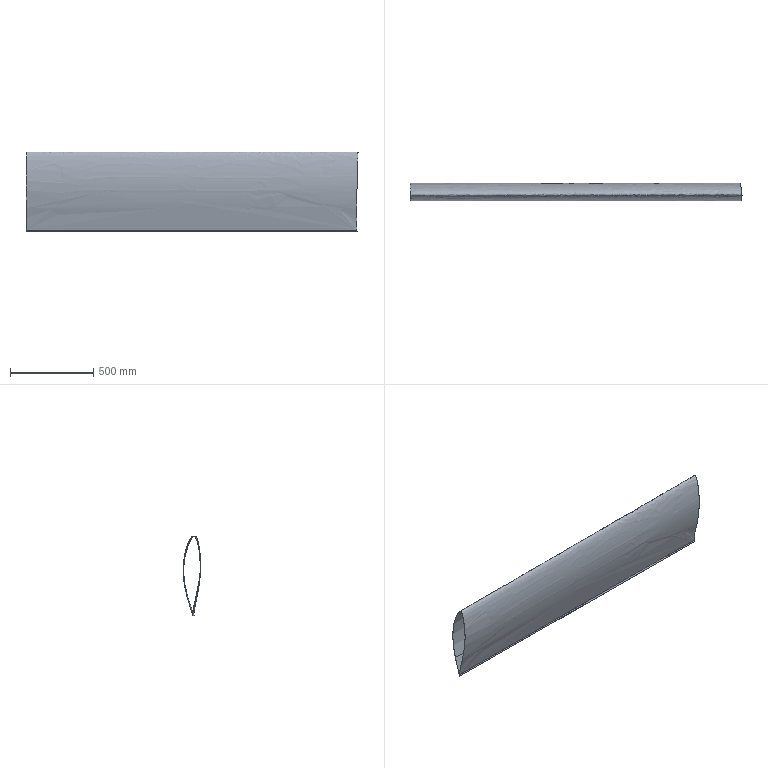Part | SolidWorks | features BaseBody 1 | 1 solid | 9 faces | box 1994 x 105.391 x 480.195 mm | volume 1098217 mm3 | spline 8 | plane 1